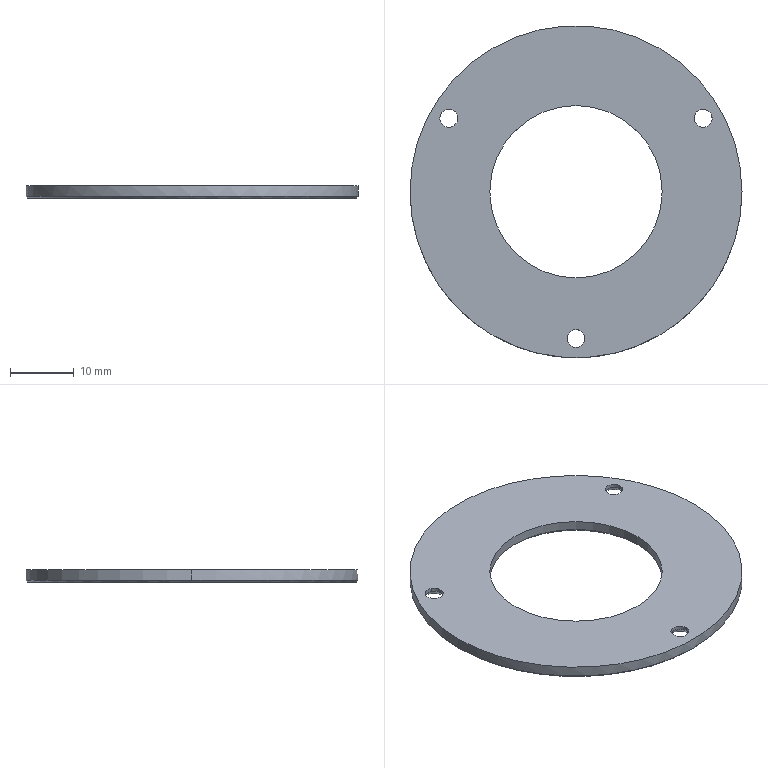Part | STEP file | TCHK-2D-D30-BB-1.stp.STEP | 1 solid | 24 faces | box 52 x 52 x 2 mm | volume 3013 mm3 | cone 12 | cylinder 10 | plane 2 | commonest cylinder face diameters 2.8 x6 27 x2 52 x2
STEP:
#1=CARTESIAN_POINT('',(14.,0.,0.000006287));
#2=VERTEX_POINT('',#1);
#3=CARTESIAN_POINT('',(-14.,0.,0.000006287));
#4=VERTEX_POINT('',#3);
#5=CARTESIAN_POINT('',(0.,0.,0.000006287));
#6=DIRECTION('',(0.,0.,1.));
#7=DIRECTION('',(1.,0.,0.));
#8=AXIS2_PLACEMENT_3D('',#5,#6,#7);
#9=CIRCLE('',#8,14.);
#10=EDGE_CURVE('',#2,#4,#9,.T.);
#11=ORIENTED_EDGE('',*,*,#10,.T.);
#12=CARTESIAN_POINT('',(0.,-14.,0.000006287));
#13=VERTEX_POINT('',#12);
#14=CARTESIAN_POINT('',(0.,0.,0.000006287));
#15=DIRECTION('',(0.,0.,1.));
#16=DIRECTION('',(-1.,0.,0.));
#17=AXIS2_PLACEMENT_3D('',#14,#15,#16);
#18=CIRCLE('',#17,14.);
#19=EDGE_CURVE('',#4,#13,#18,.T.);
#20=ORIENTED_EDGE('',*,*,#19,.T.);
#21=CARTESIAN_POINT('',(0.,0.,0.000006287));
#22=DIRECTION('',(0.,0.,1.));
#23=DIRECTION('',(-1.,0.,0.));
#24=AXIS2_PLACEMENT_3D('',#21,#22,#23);
#25=CIRCLE('',#24,14.);
#26=EDGE_CURVE('',#13,#2,#25,.T.);
#27=ORIENTED_EDGE('',*,*,#26,.T.);
#28=EDGE_LOOP('',(#11,#20,#27));
#29=FACE_BOUND('',#28,.T.);
#30=CARTESIAN_POINT('',(-0.7839,-25.688,0.));
#31=VERTEX_POINT('',#30);
#32=CARTESIAN_POINT('',(-1.4,-25.425,0.));
#33=VERTEX_POINT('',#32);
#34=CARTESIAN_POINT('',(0.,-23.,0.));
#35=DIRECTION('',(0.,0.,-1.));
#36=DIRECTION('',(-0.28,-0.96,0.));
#37=AXIS2_PLACEMENT_3D('',#34,#35,#36);
#38=CIRCLE('',#37,2.8);
#39=EDGE_CURVE('',#31,#33,#38,.T.);
#40=ORIENTED_EDGE('',*,*,#39,.F.);
#41=CARTESIAN_POINT('',(-25.7,-0.000000004,0.000001018));
#42=VERTEX_POINT('',#41);
#43=CARTESIAN_POINT('',(0.,0.,0.));
#44=DIRECTION('',(0.,0.,-1.));
#45=DIRECTION('',(-0.0305,-0.9995,0.));
#46=AXIS2_PLACEMENT_3D('',#43,#44,#45);
#47=CIRCLE('',#46,25.7);
#48=EDGE_CURVE('',#31,#42,#47,.T.);
#49=ORIENTED_EDGE('',*,*,#48,.T.);
#50=CARTESIAN_POINT('',(-22.638,12.165,0.));
#51=VERTEX_POINT('',#50);
#52=CARTESIAN_POINT('',(0.,0.,0.));
#53=DIRECTION('',(0.,0.,-1.));
#54=DIRECTION('',(-1.,0.,0.));
#55=AXIS2_PLACEMENT_3D('',#52,#53,#54);
#56=CIRCLE('',#55,25.7);
#57=EDGE_CURVE('',#42,#51,#56,.T.);
#58=ORIENTED_EDGE('',*,*,#57,.T.);
#59=CARTESIAN_POINT('',(-18.519,9.075,0.));
#60=VERTEX_POINT('',#59);
#61=CARTESIAN_POINT('',(-19.919,11.5,0.));
#62=DIRECTION('',(0.,0.,-1.));
#63=DIRECTION('',(0.5,-0.866,0.));
#64=AXIS2_PLACEMENT_3D('',#61,#62,#63);
#65=CIRCLE('',#64,2.8);
#66=EDGE_CURVE('',#60,#51,#65,.T.);
#67=ORIENTED_EDGE('',*,*,#66,.F.);
#68=CARTESIAN_POINT('',(-21.319,13.925,0.));
#69=VERTEX_POINT('',#68);
#70=CARTESIAN_POINT('',(-19.919,11.5,0.));
#71=DIRECTION('',(0.,0.,-1.));
#72=DIRECTION('',(-0.5,0.866,0.));
#73=AXIS2_PLACEMENT_3D('',#70,#71,#72);
#74=CIRCLE('',#73,2.8);
#75=EDGE_CURVE('',#69,#60,#74,.T.);
#76=ORIENTED_EDGE('',*,*,#75,.F.);
#77=CARTESIAN_POINT('',(-21.855,13.523,0.));
#78=VERTEX_POINT('',#77);
#79=CARTESIAN_POINT('',(-19.919,11.5,0.));
#80=DIRECTION('',(0.,0.,-1.));
#81=DIRECTION('',(-0.6914,0.7225,0.));
#82=AXIS2_PLACEMENT_3D('',#79,#80,#81);
#83=CIRCLE('',#82,2.8);
#84=EDGE_CURVE('',#78,#69,#83,.T.);
#85=ORIENTED_EDGE('',*,*,#84,.F.);
#86=CARTESIAN_POINT('',(21.855,13.523,0.));
#87=VERTEX_POINT('',#86);
#88=CARTESIAN_POINT('',(0.,0.,0.));
#89=DIRECTION('',(0.,0.,-1.));
#90=DIRECTION('',(-0.8504,0.5262,0.));
#91=AXIS2_PLACEMENT_3D('',#88,#89,#90);
#92=CIRCLE('',#91,25.7);
#93=EDGE_CURVE('',#78,#87,#92,.T.);
#94=ORIENTED_EDGE('',*,*,#93,.T.);
#95=CARTESIAN_POINT('',(17.119,11.5,0.));
#96=VERTEX_POINT('',#95);
#97=CARTESIAN_POINT('',(19.919,11.5,0.));
#98=DIRECTION('',(0.,0.,-1.));
#99=DIRECTION('',(-1.,0.,0.));
#100=AXIS2_PLACEMENT_3D('',#97,#98,#99);
#101=CIRCLE('',#100,2.8);
#102=EDGE_CURVE('',#96,#87,#101,.T.);
#103=ORIENTED_EDGE('',*,*,#102,.F.);
#104=CARTESIAN_POINT('',(22.719,11.5,0.));
#105=VERTEX_POINT('',#104);
#106=CARTESIAN_POINT('',(19.919,11.5,0.));
#107=DIRECTION('',(0.,0.,-1.));
#108=DIRECTION('',(1.,0.,0.));
#109=AXIS2_PLACEMENT_3D('',#106,#107,#108);
#110=CIRCLE('',#109,2.8);
#111=EDGE_CURVE('',#105,#96,#110,.T.);
#112=ORIENTED_EDGE('',*,*,#111,.F.);
#113=CARTESIAN_POINT('',(22.638,12.165,0.));
#114=VERTEX_POINT('',#113);
#115=CARTESIAN_POINT('',(19.919,11.5,0.));
#116=DIRECTION('',(0.,0.,-1.));
#117=DIRECTION('',(0.9714,0.2376,0.));
#118=AXIS2_PLACEMENT_3D('',#115,#116,#117);
#119=CIRCLE('',#118,2.8);
#120=EDGE_CURVE('',#114,#105,#119,.T.);
#121=ORIENTED_EDGE('',*,*,#120,.F.);
#122=CARTESIAN_POINT('',(25.7,0.000000004,0.000001018));
#123=VERTEX_POINT('',#122);
#124=CARTESIAN_POINT('',(0.,0.,0.));
#125=DIRECTION('',(0.,0.,-1.));
#126=DIRECTION('',(0.8809,0.4734,0.));
#127=AXIS2_PLACEMENT_3D('',#124,#125,#126);
#128=CIRCLE('',#127,25.7);
#129=EDGE_CURVE('',#114,#123,#128,.T.);
#130=ORIENTED_EDGE('',*,*,#129,.T.);
#131=CARTESIAN_POINT('',(0.7839,-25.688,0.));
#132=VERTEX_POINT('',#131);
#133=CARTESIAN_POINT('',(0.,0.,0.));
#134=DIRECTION('',(0.,0.,-1.));
#135=DIRECTION('',(1.,0.,0.));
#136=AXIS2_PLACEMENT_3D('',#133,#134,#135);
#137=CIRCLE('',#136,25.7);
#138=EDGE_CURVE('',#123,#132,#137,.T.);
#139=ORIENTED_EDGE('',*,*,#138,.T.);
#140=CARTESIAN_POINT('',(1.4,-20.575,0.));
#141=VERTEX_POINT('',#140);
#142=CARTESIAN_POINT('',(0.,-23.,0.));
#143=DIRECTION('',(0.,0.,-1.));
#144=DIRECTION('',(0.5,0.866,0.));
#145=AXIS2_PLACEMENT_3D('',#142,#143,#144);
#146=CIRCLE('',#145,2.8);
#147=EDGE_CURVE('',#141,#132,#146,.T.);
#148=ORIENTED_EDGE('',*,*,#147,.F.);
#149=CARTESIAN_POINT('',(0.,-23.,0.));
#150=DIRECTION('',(0.,0.,-1.));
#151=DIRECTION('',(-0.5,-0.866,0.));
#152=AXIS2_PLACEMENT_3D('',#149,#150,#151);
#153=CIRCLE('',#152,2.8);
#154=EDGE_CURVE('',#33,#141,#153,.T.);
#155=ORIENTED_EDGE('',*,*,#154,.F.);
#156=EDGE_LOOP('',(#40,#49,#58,#67,#76,#85,#94,#103,#112,#121,#130,#139,#148,#155));
#157=FACE_OUTER_BOUND('',#156,.T.);
#158=CARTESIAN_POINT('',(0.,0.,0.));
#159=DIRECTION('',(0.,0.,1.));
#160=DIRECTION('',(1.,0.,0.));
#161=AXIS2_PLACEMENT_3D('',#158,#159,#160);
#162=PLANE('',#161);
#163=ADVANCED_FACE('',(#29,#157),#162,.F.);
#164=CARTESIAN_POINT('',(0.,-13.5,0.5));
#165=VERTEX_POINT('',#164);
#166=CARTESIAN_POINT('',(0.,-13.75,0.25));
#167=DIRECTION('',(0.,-0.7071,-0.7071));
#168=VECTOR('',#167,1000.);
#169=LINE('',#166,#168);
#170=EDGE_CURVE('',#165,#13,#169,.T.);
#171=ORIENTED_EDGE('',*,*,#170,.F.);
#172=CARTESIAN_POINT('',(13.5,0.,0.5));
#173=VERTEX_POINT('',#172);
#174=CARTESIAN_POINT('',(0.,0.,0.5));
#175=DIRECTION('',(0.,0.,1.));
#176=DIRECTION('',(-1.,0.,0.));
#177=AXIS2_PLACEMENT_3D('',#174,#175,#176);
#178=CIRCLE('',#177,13.5);
#179=EDGE_CURVE('',#165,#173,#178,.T.);
#180=ORIENTED_EDGE('',*,*,#179,.T.);
#181=CARTESIAN_POINT('',(14.,0.000000008,0.000002614));
#182=DIRECTION('',(-0.7071,-0.000000003,0.7071));
#183=VECTOR('',#182,1000.);
#184=LINE('',#181,#183);
#185=EDGE_CURVE('',#2,#173,#184,.T.);
#186=ORIENTED_EDGE('',*,*,#185,.F.);
#187=ORIENTED_EDGE('',*,*,#26,.F.);
#188=EDGE_LOOP('',(#171,#180,#186,#187));
#189=FACE_OUTER_BOUND('',#188,.T.);
#190=CARTESIAN_POINT('',(0.,0.,0.25));
#191=DIRECTION('',(0.,0.,-1.));
#192=DIRECTION('',(0.,-1.,0.));
#193=AXIS2_PLACEMENT_3D('',#190,#191,#192);
#194=CONICAL_SURFACE('',#193,13.75,0.7854);
#195=ADVANCED_FACE('',(#189),#194,.F.);
#196=ORIENTED_EDGE('',*,*,#185,.T.);
#197=CARTESIAN_POINT('',(-13.5,0.,0.5));
#198=VERTEX_POINT('',#197);
#199=CARTESIAN_POINT('',(0.,0.,0.5));
#200=DIRECTION('',(0.,0.,1.));
#201=DIRECTION('',(1.,0.,0.));
#202=AXIS2_PLACEMENT_3D('',#199,#200,#201);
#203=CIRCLE('',#202,13.5);
#204=EDGE_CURVE('',#173,#198,#203,.T.);
#205=ORIENTED_EDGE('',*,*,#204,.T.);
#206=CARTESIAN_POINT('',(-14.,-0.000000008,0.000002614));
#207=DIRECTION('',(0.7071,0.000000003,0.7071));
#208=VECTOR('',#207,1000.);
#209=LINE('',#206,#208);
#210=EDGE_CURVE('',#4,#198,#209,.T.);
#211=ORIENTED_EDGE('',*,*,#210,.F.);
#212=ORIENTED_EDGE('',*,*,#10,.F.);
#213=EDGE_LOOP('',(#196,#205,#211,#212));
#214=FACE_OUTER_BOUND('',#213,.T.);
#215=CARTESIAN_POINT('',(0.,0.,0.25));
#216=DIRECTION('',(0.,0.,-1.));
#217=DIRECTION('',(0.,-1.,0.));
#218=AXIS2_PLACEMENT_3D('',#215,#216,#217);
#219=CONICAL_SURFACE('',#218,13.75,0.7854);
#220=ADVANCED_FACE('',(#214),#219,.F.);
#221=CARTESIAN_POINT('',(13.5,0.,2.));
#222=VERTEX_POINT('',#221);
#223=CARTESIAN_POINT('',(13.5,0.,2.));
#224=DIRECTION('',(0.00000126,0.000000004,-1.));
#225=VECTOR('',#224,1000.);
#226=LINE('',#223,#225);
#227=EDGE_CURVE('',#222,#173,#226,.T.);
#228=ORIENTED_EDGE('',*,*,#227,.F.);
#229=CARTESIAN_POINT('',(-13.5,0.,2.));
#230=VERTEX_POINT('',#229);
#231=CARTESIAN_POINT('',(0.,0.,2.));
#232=DIRECTION('',(0.,0.,1.));
#233=DIRECTION('',(1.,0.,0.));
#234=AXIS2_PLACEMENT_3D('',#231,#232,#233);
#235=CIRCLE('',#234,13.5);
#236=EDGE_CURVE('',#222,#230,#235,.T.);
#237=ORIENTED_EDGE('',*,*,#236,.T.);
#238=CARTESIAN_POINT('',(-13.5,0.,2.));
#239=DIRECTION('',(-0.00000126,-0.000000004,-1.));
#240=VECTOR('',#239,1000.);
#241=LINE('',#238,#240);
#242=EDGE_CURVE('',#230,#198,#241,.T.);
#243=ORIENTED_EDGE('',*,*,#242,.T.);
#244=ORIENTED_EDGE('',*,*,#204,.F.);
#245=EDGE_LOOP('',(#228,#237,#243,#244));
#246=FACE_OUTER_BOUND('',#245,.T.);
#247=CARTESIAN_POINT('',(0.,0.,2.));
#248=DIRECTION('',(0.,0.,1.));
#249=DIRECTION('',(1.,0.,0.));
#250=AXIS2_PLACEMENT_3D('',#247,#248,#249);
#251=CYLINDRICAL_SURFACE('',#250,13.5);
#252=ADVANCED_FACE('',(#246),#251,.F.);
#253=ORIENTED_EDGE('',*,*,#242,.F.);
#254=CARTESIAN_POINT('',(0.,0.,2.));
#255=DIRECTION('',(0.,0.,1.));
#256=DIRECTION('',(-1.,0.,0.));
#257=AXIS2_PLACEMENT_3D('',#254,#255,#256);
#258=CIRCLE('',#257,13.5);
#259=EDGE_CURVE('',#230,#222,#258,.T.);
#260=ORIENTED_EDGE('',*,*,#259,.T.);
#261=ORIENTED_EDGE('',*,*,#227,.T.);
#262=ORIENTED_EDGE('',*,*,#179,.F.);
#263=CARTESIAN_POINT('',(0.,0.,0.5));
#264=DIRECTION('',(0.,0.,1.));
#265=DIRECTION('',(-1.,0.,0.));
#266=AXIS2_PLACEMENT_3D('',#263,#264,#265);
#267=CIRCLE('',#266,13.5);
#268=EDGE_CURVE('',#198,#165,#267,.T.);
#269=ORIENTED_EDGE('',*,*,#268,.F.);
#270=EDGE_LOOP('',(#253,#260,#261,#262,#269));
#271=FACE_OUTER_BOUND('',#270,.T.);
#272=CARTESIAN_POINT('',(0.,0.,2.));
#273=DIRECTION('',(0.,0.,1.));
#274=DIRECTION('',(1.,0.,0.));
#275=AXIS2_PLACEMENT_3D('',#272,#273,#274);
#276=CYLINDRICAL_SURFACE('',#275,13.5);
#277=ADVANCED_FACE('',(#271),#276,.F.);
#278=CARTESIAN_POINT('',(1.4,-23.,2.));
#279=VERTEX_POINT('',#278);
#280=CARTESIAN_POINT('',(-1.4,-23.,2.));
#281=VERTEX_POINT('',#280);
#282=CARTESIAN_POINT('',(0.,-23.,2.));
#283=DIRECTION('',(0.,0.,-1.));
#284=DIRECTION('',(1.,0.,0.));
#285=AXIS2_PLACEMENT_3D('',#282,#283,#284);
#286=CIRCLE('',#285,1.4);
#287=EDGE_CURVE('',#279,#281,#286,.T.);
#288=ORIENTED_EDGE('',*,*,#287,.T.);
#289=CARTESIAN_POINT('',(0.,-23.,2.));
#290=DIRECTION('',(0.,0.,-1.));
#291=DIRECTION('',(-1.,0.,0.));
#292=AXIS2_PLACEMENT_3D('',#289,#290,#291);
#293=CIRCLE('',#292,1.4);
#294=EDGE_CURVE('',#281,#279,#293,.T.);
#295=ORIENTED_EDGE('',*,*,#294,.T.);
#296=EDGE_LOOP('',(#288,#295));
#297=FACE_BOUND('',#296,.T.);
#298=CARTESIAN_POINT('',(19.219,12.712,2.));
#299=VERTEX_POINT('',#298);
#300=CARTESIAN_POINT('',(20.619,10.288,2.));
#301=VERTEX_POINT('',#300);
#302=CARTESIAN_POINT('',(19.919,11.5,2.));
#303=DIRECTION('',(0.,0.,-1.));
#304=DIRECTION('',(-0.5,0.866,0.));
#305=AXIS2_PLACEMENT_3D('',#302,#303,#304);
#306=CIRCLE('',#305,1.4);
#307=EDGE_CURVE('',#299,#301,#306,.T.);
#308=ORIENTED_EDGE('',*,*,#307,.T.);
#309=CARTESIAN_POINT('',(19.919,11.5,2.));
#310=DIRECTION('',(0.,0.,-1.));
#311=DIRECTION('',(0.5,-0.866,0.));
#312=AXIS2_PLACEMENT_3D('',#309,#310,#311);
#313=CIRCLE('',#312,1.4);
#314=EDGE_CURVE('',#301,#299,#313,.T.);
#315=ORIENTED_EDGE('',*,*,#314,.T.);
#316=EDGE_LOOP('',(#308,#315));
#317=FACE_BOUND('',#316,.T.);
#318=CARTESIAN_POINT('',(-20.619,10.288,2.));
#319=VERTEX_POINT('',#318);
#320=CARTESIAN_POINT('',(-19.219,12.712,2.));
#321=VERTEX_POINT('',#320);
#322=CARTESIAN_POINT('',(-19.919,11.5,2.));
#323=DIRECTION('',(0.,0.,-1.));
#324=DIRECTION('',(-0.5,-0.866,0.));
#325=AXIS2_PLACEMENT_3D('',#322,#323,#324);
#326=CIRCLE('',#325,1.4);
#327=EDGE_CURVE('',#319,#321,#326,.T.);
#328=ORIENTED_EDGE('',*,*,#327,.T.);
#329=CARTESIAN_POINT('',(-19.919,11.5,2.));
#330=DIRECTION('',(0.,0.,-1.));
#331=DIRECTION('',(0.5,0.866,0.));
#332=AXIS2_PLACEMENT_3D('',#329,#330,#331);
#333=CIRCLE('',#332,1.4);
#334=EDGE_CURVE('',#321,#319,#333,.T.);
#335=ORIENTED_EDGE('',*,*,#334,.T.);
#336=EDGE_LOOP('',(#328,#335));
#337=FACE_BOUND('',#336,.T.);
#338=ORIENTED_EDGE('',*,*,#259,.F.);
#339=ORIENTED_EDGE('',*,*,#236,.F.);
#340=EDGE_LOOP('',(#338,#339));
#341=FACE_BOUND('',#340,.T.);
#342=CARTESIAN_POINT('',(-26.,0.,2.));
#343=VERTEX_POINT('',#342);
#344=CARTESIAN_POINT('',(26.,0.,2.));
#345=VERTEX_POINT('',#344);
#346=CARTESIAN_POINT('',(0.,0.,2.));
#347=DIRECTION('',(0.,0.,1.));
#348=DIRECTION('',(-1.,0.,0.));
#349=AXIS2_PLACEMENT_3D('',#346,#347,#348);
#350=CIRCLE('',#349,26.);
#351=EDGE_CURVE('',#343,#345,#350,.T.);
#352=ORIENTED_EDGE('',*,*,#351,.T.);
#353=CARTESIAN_POINT('',(0.,0.,2.));
#354=DIRECTION('',(0.,0.,1.));
#355=DIRECTION('',(1.,0.,0.));
#356=AXIS2_PLACEMENT_3D('',#353,#354,#355);
#357=CIRCLE('',#356,26.);
#358=EDGE_CURVE('',#345,#343,#357,.T.);
#359=ORIENTED_EDGE('',*,*,#358,.T.);
#360=EDGE_LOOP('',(#352,#359));
#361=FACE_OUTER_BOUND('',#360,.T.);
#362=CARTESIAN_POINT('',(0.,0.,2.));
#363=DIRECTION('',(0.,0.,1.));
#364=DIRECTION('',(1.,0.,0.));
#365=AXIS2_PLACEMENT_3D('',#362,#363,#364);
#366=PLANE('',#365);
#367=ADVANCED_FACE('',(#297,#317,#337,#341,#361),#366,.T.);
#368=CARTESIAN_POINT('',(-26.,0.,0.3));
#369=VERTEX_POINT('',#368);
#370=CARTESIAN_POINT('',(-26.,-0.000000003,0.3));
#371=DIRECTION('',(-0.000000455,0.000000002,1.));
#372=VECTOR('',#371,1000.);
#373=LINE('',#370,#372);
#374=EDGE_CURVE('',#369,#343,#373,.T.);
#375=ORIENTED_EDGE('',*,*,#374,.T.);
#376=ORIENTED_EDGE('',*,*,#358,.F.);
#377=CARTESIAN_POINT('',(26.,0.,0.3));
#378=VERTEX_POINT('',#377);
#379=CARTESIAN_POINT('',(26.,0.000000003,0.3));
#380=DIRECTION('',(0.000000455,-0.000000002,1.));
#381=VECTOR('',#380,1000.);
#382=LINE('',#379,#381);
#383=EDGE_CURVE('',#378,#345,#382,.T.);
#384=ORIENTED_EDGE('',*,*,#383,.F.);
#385=CARTESIAN_POINT('',(0.,0.,0.3));
#386=DIRECTION('',(0.,0.,-1.));
#387=DIRECTION('',(-1.,0.,0.));
#388=AXIS2_PLACEMENT_3D('',#385,#386,#387);
#389=CIRCLE('',#388,26.);
#390=EDGE_CURVE('',#369,#378,#389,.T.);
#391=ORIENTED_EDGE('',*,*,#390,.F.);
#392=EDGE_LOOP('',(#375,#376,#384,#391));
#393=FACE_OUTER_BOUND('',#392,.T.);
#394=CARTESIAN_POINT('',(0.,0.,0.));
#395=DIRECTION('',(0.,0.,1.));
#396=DIRECTION('',(1.,0.,0.));
#397=AXIS2_PLACEMENT_3D('',#394,#395,#396);
#398=CYLINDRICAL_SURFACE('',#397,26.);
#399=ADVANCED_FACE('',(#393),#398,.T.);
#400=ORIENTED_EDGE('',*,*,#57,.F.);
#401=CARTESIAN_POINT('',(-25.7,-0.000000004,0.000001018));
#402=DIRECTION('',(-0.7071,0.000000002,0.7071));
#403=VECTOR('',#402,1000.);
#404=LINE('',#401,#403);
#405=EDGE_CURVE('',#42,#369,#404,.T.);
#406=ORIENTED_EDGE('',*,*,#405,.T.);
#407=ORIENTED_EDGE('',*,*,#390,.T.);
#408=CARTESIAN_POINT('',(25.7,0.000000004,0.000001018));
#409=DIRECTION('',(0.7071,-0.000000002,0.7071));
#410=VECTOR('',#409,1000.);
#411=LINE('',#408,#410);
#412=EDGE_CURVE('',#123,#378,#411,.T.);
#413=ORIENTED_EDGE('',*,*,#412,.F.);
#414=ORIENTED_EDGE('',*,*,#129,.F.);
#415=CARTESIAN_POINT('',(22.638,12.165,0.));
#416=CARTESIAN_POINT('',(22.45,12.657,0.06653));
#417=CARTESIAN_POINT('',(22.186,13.113,0.06653));
#418=CARTESIAN_POINT('',(21.855,13.523,0.));
#419=B_SPLINE_CURVE_WITH_KNOTS('',3,(#415,#416,#417,#418),.UNSPECIFIED.,.F.,.F.,(4,4),(0.,1.),.UNSPECIFIED.);
#420=EDGE_CURVE('',#114,#87,#419,.T.);
#421=ORIENTED_EDGE('',*,*,#420,.T.);
#422=ORIENTED_EDGE('',*,*,#93,.F.);
#423=CARTESIAN_POINT('',(-21.855,13.523,0.));
#424=CARTESIAN_POINT('',(-22.186,13.113,0.06653));
#425=CARTESIAN_POINT('',(-22.45,12.657,0.06653));
#426=CARTESIAN_POINT('',(-22.638,12.165,0.));
#427=B_SPLINE_CURVE_WITH_KNOTS('',3,(#423,#424,#425,#426),.UNSPECIFIED.,.F.,.F.,(4,4),(0.,1.),.UNSPECIFIED.);
#428=EDGE_CURVE('',#78,#51,#427,.T.);
#429=ORIENTED_EDGE('',*,*,#428,.T.);
#430=EDGE_LOOP('',(#400,#406,#407,#413,#414,#421,#422,#429));
#431=FACE_OUTER_BOUND('',#430,.T.);
#432=CARTESIAN_POINT('',(0.,0.,0.15));
#433=DIRECTION('',(0.,0.,1.));
#434=DIRECTION('',(0.,-1.,0.));
#435=AXIS2_PLACEMENT_3D('',#432,#433,#434);
#436=CONICAL_SURFACE('',#435,25.85,0.7854);
#437=ADVANCED_FACE('',(#431),#436,.T.);
#438=ORIENTED_EDGE('',*,*,#428,.F.);
#439=ORIENTED_EDGE('',*,*,#84,.T.);
#440=CARTESIAN_POINT('',(-20.619,12.712,1.4));
#441=VERTEX_POINT('',#440);
#442=CARTESIAN_POINT('',(-21.319,13.925,0.));
#443=DIRECTION('',(0.3536,-0.6124,0.7071));
#444=VECTOR('',#443,1000.);
#445=LINE('',#442,#444);
#446=EDGE_CURVE('',#69,#441,#445,.T.);
#447=ORIENTED_EDGE('',*,*,#446,.T.);
#448=CARTESIAN_POINT('',(-20.619,10.288,1.4));
#449=VERTEX_POINT('',#448);
#450=CARTESIAN_POINT('',(-19.919,11.5,1.4));
#451=DIRECTION('',(0.,0.,-1.));
#452=DIRECTION('',(-0.5,-0.866,0.));
#453=AXIS2_PLACEMENT_3D('',#450,#451,#452);
#454=CIRCLE('',#453,1.4);
#455=EDGE_CURVE('',#449,#441,#454,.T.);
#456=ORIENTED_EDGE('',*,*,#455,.F.);
#457=CARTESIAN_POINT('',(-19.219,10.288,1.4));
#458=VERTEX_POINT('',#457);
#459=CARTESIAN_POINT('',(-19.919,11.5,1.4));
#460=DIRECTION('',(0.,0.,-1.));
#461=DIRECTION('',(0.5,-0.866,0.));
#462=AXIS2_PLACEMENT_3D('',#459,#460,#461);
#463=CIRCLE('',#462,1.4);
#464=EDGE_CURVE('',#458,#449,#463,.T.);
#465=ORIENTED_EDGE('',*,*,#464,.F.);
#466=CARTESIAN_POINT('',(-18.519,9.075,0.));
#467=DIRECTION('',(-0.3536,0.6124,0.7071));
#468=VECTOR('',#467,1000.);
#469=LINE('',#466,#468);
#470=EDGE_CURVE('',#60,#458,#469,.T.);
#471=ORIENTED_EDGE('',*,*,#470,.F.);
#472=ORIENTED_EDGE('',*,*,#66,.T.);
#473=EDGE_LOOP('',(#438,#439,#447,#456,#465,#471,#472));
#474=FACE_OUTER_BOUND('',#473,.T.);
#475=CARTESIAN_POINT('',(-19.919,11.5,0.7));
#476=DIRECTION('',(0.,0.,-1.));
#477=DIRECTION('',(0.5,-0.866,0.));
#478=AXIS2_PLACEMENT_3D('',#475,#476,#477);
#479=CONICAL_SURFACE('',#478,2.1,0.7854);
#480=ADVANCED_FACE('',(#474),#479,.F.);
#481=ORIENTED_EDGE('',*,*,#470,.T.);
#482=CARTESIAN_POINT('',(-19.219,12.712,1.4));
#483=VERTEX_POINT('',#482);
#484=CARTESIAN_POINT('',(-19.919,11.5,1.4));
#485=DIRECTION('',(0.,0.,-1.));
#486=DIRECTION('',(0.5,0.866,0.));
#487=AXIS2_PLACEMENT_3D('',#484,#485,#486);
#488=CIRCLE('',#487,1.4);
#489=EDGE_CURVE('',#483,#458,#488,.T.);
#490=ORIENTED_EDGE('',*,*,#489,.F.);
#491=CARTESIAN_POINT('',(-19.919,11.5,1.4));
#492=DIRECTION('',(0.,0.,-1.));
#493=DIRECTION('',(-0.5,0.866,0.));
#494=AXIS2_PLACEMENT_3D('',#491,#492,#493);
#495=CIRCLE('',#494,1.4);
#496=EDGE_CURVE('',#441,#483,#495,.T.);
#497=ORIENTED_EDGE('',*,*,#496,.F.);
#498=ORIENTED_EDGE('',*,*,#446,.F.);
#499=ORIENTED_EDGE('',*,*,#75,.T.);
#500=EDGE_LOOP('',(#481,#490,#497,#498,#499));
#501=FACE_OUTER_BOUND('',#500,.T.);
#502=CARTESIAN_POINT('',(-19.919,11.5,0.7));
#503=DIRECTION('',(0.,0.,-1.));
#504=DIRECTION('',(0.5,-0.866,0.));
#505=AXIS2_PLACEMENT_3D('',#502,#503,#504);
#506=CONICAL_SURFACE('',#505,2.1,0.7854);
#507=ADVANCED_FACE('',(#501),#506,.F.);
#508=CARTESIAN_POINT('',(-19.219,12.712,2.));
#509=DIRECTION('',(0.,0.,-1.));
#510=VECTOR('',#509,1000.);
#511=LINE('',#508,#510);
#512=EDGE_CURVE('',#321,#483,#511,.T.);
#513=ORIENTED_EDGE('',*,*,#512,.F.);
#514=ORIENTED_EDGE('',*,*,#327,.F.);
#515=CARTESIAN_POINT('',(-20.619,10.288,2.));
#516=DIRECTION('',(0.,0.,-1.));
#517=VECTOR('',#516,1000.);
#518=LINE('',#515,#517);
#519=EDGE_CURVE('',#319,#449,#518,.T.);
#520=ORIENTED_EDGE('',*,*,#519,.T.);
#521=ORIENTED_EDGE('',*,*,#455,.T.);
#522=ORIENTED_EDGE('',*,*,#496,.T.);
#523=EDGE_LOOP('',(#513,#514,#520,#521,#522));
#524=FACE_OUTER_BOUND('',#523,.T.);
#525=CARTESIAN_POINT('',(-19.919,11.5,2.));
#526=DIRECTION('',(0.,0.,-1.));
#527=DIRECTION('',(0.5,0.866,0.));
#528=AXIS2_PLACEMENT_3D('',#525,#526,#527);
#529=CYLINDRICAL_SURFACE('',#528,1.4);
#530=ADVANCED_FACE('',(#524),#529,.F.);
#531=ORIENTED_EDGE('',*,*,#464,.T.);
#532=ORIENTED_EDGE('',*,*,#519,.F.);
#533=ORIENTED_EDGE('',*,*,#334,.F.);
#534=ORIENTED_EDGE('',*,*,#512,.T.);
#535=ORIENTED_EDGE('',*,*,#489,.T.);
#536=EDGE_LOOP('',(#531,#532,#533,#534,#535));
#537=FACE_OUTER_BOUND('',#536,.T.);
#538=CARTESIAN_POINT('',(-19.919,11.5,2.));
#539=DIRECTION('',(0.,0.,-1.));
#540=DIRECTION('',(0.5,0.866,0.));
#541=AXIS2_PLACEMENT_3D('',#538,#539,#540);
#542=CYLINDRICAL_SURFACE('',#541,1.4);
#543=ADVANCED_FACE('',(#537),#542,.F.);
#544=ORIENTED_EDGE('',*,*,#420,.F.);
#545=ORIENTED_EDGE('',*,*,#120,.T.);
#546=CARTESIAN_POINT('',(21.319,11.5,1.4));
#547=VERTEX_POINT('',#546);
#548=CARTESIAN_POINT('',(22.719,11.5,0.));
#549=DIRECTION('',(-0.7071,0.,0.7071));
#550=VECTOR('',#549,1000.);
#551=LINE('',#548,#550);
#552=EDGE_CURVE('',#105,#547,#551,.T.);
#553=ORIENTED_EDGE('',*,*,#552,.T.);
#554=CARTESIAN_POINT('',(19.219,12.712,1.4));
#555=VERTEX_POINT('',#554);
#556=CARTESIAN_POINT('',(19.919,11.5,1.4));
#557=DIRECTION('',(0.,0.,-1.));
#558=DIRECTION('',(-0.5,0.866,0.));
#559=AXIS2_PLACEMENT_3D('',#556,#557,#558);
#560=CIRCLE('',#559,1.4);
#561=EDGE_CURVE('',#555,#547,#560,.T.);
#562=ORIENTED_EDGE('',*,*,#561,.F.);
#563=CARTESIAN_POINT('',(18.519,11.5,1.4));
#564=VERTEX_POINT('',#563);
#565=CARTESIAN_POINT('',(19.919,11.5,1.4));
#566=DIRECTION('',(0.,0.,-1.));
#567=DIRECTION('',(-1.,0.,0.));
#568=AXIS2_PLACEMENT_3D('',#565,#566,#567);
#569=CIRCLE('',#568,1.4);
#570=EDGE_CURVE('',#564,#555,#569,.T.);
#571=ORIENTED_EDGE('',*,*,#570,.F.);
#572=CARTESIAN_POINT('',(17.119,11.5,0.));
#573=DIRECTION('',(0.7071,0.,0.7071));
#574=VECTOR('',#573,1000.);
#575=LINE('',#572,#574);
#576=EDGE_CURVE('',#96,#564,#575,.T.);
#577=ORIENTED_EDGE('',*,*,#576,.F.);
#578=ORIENTED_EDGE('',*,*,#102,.T.);
#579=EDGE_LOOP('',(#544,#545,#553,#562,#571,#577,#578));
#580=FACE_OUTER_BOUND('',#579,.T.);
#581=CARTESIAN_POINT('',(19.919,11.5,0.7));
#582=DIRECTION('',(0.,0.,-1.));
#583=DIRECTION('',(-1.,0.,0.));
#584=AXIS2_PLACEMENT_3D('',#581,#582,#583);
#585=CONICAL_SURFACE('',#584,2.1,0.7854);
#586=ADVANCED_FACE('',(#580),#585,.F.);
#587=ORIENTED_EDGE('',*,*,#576,.T.);
#588=CARTESIAN_POINT('',(20.619,10.288,1.4));
#589=VERTEX_POINT('',#588);
#590=CARTESIAN_POINT('',(19.919,11.5,1.4));
#591=DIRECTION('',(0.,0.,-1.));
#592=DIRECTION('',(0.5,-0.866,0.));
#593=AXIS2_PLACEMENT_3D('',#590,#591,#592);
#594=CIRCLE('',#593,1.4);
#595=EDGE_CURVE('',#589,#564,#594,.T.);
#596=ORIENTED_EDGE('',*,*,#595,.F.);
#597=CARTESIAN_POINT('',(19.919,11.5,1.4));
#598=DIRECTION('',(0.,0.,-1.));
#599=DIRECTION('',(1.,0.,0.));
#600=AXIS2_PLACEMENT_3D('',#597,#598,#599);
#601=CIRCLE('',#600,1.4);
#602=EDGE_CURVE('',#547,#589,#601,.T.);
#603=ORIENTED_EDGE('',*,*,#602,.F.);
#604=ORIENTED_EDGE('',*,*,#552,.F.);
#605=ORIENTED_EDGE('',*,*,#111,.T.);
#606=EDGE_LOOP('',(#587,#596,#603,#604,#605));
#607=FACE_OUTER_BOUND('',#606,.T.);
#608=CARTESIAN_POINT('',(19.919,11.5,0.7));
#609=DIRECTION('',(0.,0.,-1.));
#610=DIRECTION('',(-1.,0.,0.));
#611=AXIS2_PLACEMENT_3D('',#608,#609,#610);
#612=CONICAL_SURFACE('',#611,2.1,0.7854);
#613=ADVANCED_FACE('',(#607),#612,.F.);
#614=CARTESIAN_POINT('',(20.619,10.288,2.));
#615=DIRECTION('',(0.,0.,-1.));
#616=VECTOR('',#615,1000.);
#617=LINE('',#614,#616);
#618=EDGE_CURVE('',#301,#589,#617,.T.);
#619=ORIENTED_EDGE('',*,*,#618,.F.);
#620=ORIENTED_EDGE('',*,*,#307,.F.);
#621=CARTESIAN_POINT('',(19.219,12.712,2.));
#622=DIRECTION('',(0.,0.,-1.));
#623=VECTOR('',#622,1000.);
#624=LINE('',#621,#623);
#625=EDGE_CURVE('',#299,#555,#624,.T.);
#626=ORIENTED_EDGE('',*,*,#625,.T.);
#627=ORIENTED_EDGE('',*,*,#561,.T.);
#628=ORIENTED_EDGE('',*,*,#602,.T.);
#629=EDGE_LOOP('',(#619,#620,#626,#627,#628));
#630=FACE_OUTER_BOUND('',#629,.T.);
#631=CARTESIAN_POINT('',(19.919,11.5,2.));
#632=DIRECTION('',(0.,0.,-1.));
#633=DIRECTION('',(0.5,-0.866,0.));
#634=AXIS2_PLACEMENT_3D('',#631,#632,#633);
#635=CYLINDRICAL_SURFACE('',#634,1.4);
#636=ADVANCED_FACE('',(#630),#635,.F.);
#637=ORIENTED_EDGE('',*,*,#570,.T.);
#638=ORIENTED_EDGE('',*,*,#625,.F.);
#639=ORIENTED_EDGE('',*,*,#314,.F.);
#640=ORIENTED_EDGE('',*,*,#618,.T.);
#641=ORIENTED_EDGE('',*,*,#595,.T.);
#642=EDGE_LOOP('',(#637,#638,#639,#640,#641));
#643=FACE_OUTER_BOUND('',#642,.T.);
#644=CARTESIAN_POINT('',(19.919,11.5,2.));
#645=DIRECTION('',(0.,0.,-1.));
#646=DIRECTION('',(0.5,-0.866,0.));
#647=AXIS2_PLACEMENT_3D('',#644,#645,#646);
#648=CYLINDRICAL_SURFACE('',#647,1.4);
#649=ADVANCED_FACE('',(#643),#648,.F.);
#650=CARTESIAN_POINT('',(0.000000009,-25.75,0.05));
#651=VERTEX_POINT('',#650);
#652=CARTESIAN_POINT('',(0.,-26.,0.3));
#653=VERTEX_POINT('',#652);
#654=CARTESIAN_POINT('',(0.,-25.85,0.15));
#655=DIRECTION('',(0.,-0.7071,0.7071));
#656=VECTOR('',#655,1000.);
#657=LINE('',#654,#656);
#658=EDGE_CURVE('',#651,#653,#657,.T.);
#659=ORIENTED_EDGE('',*,*,#658,.F.);
#660=CARTESIAN_POINT('',(0.000000009,-25.75,0.05));
#661=CARTESIAN_POINT('',(0.2613,-25.75,0.05001));
#662=CARTESIAN_POINT('',(0.5231,-25.729,0.03334));
#663=CARTESIAN_POINT('',(0.7839,-25.688,0.));
#664=B_SPLINE_CURVE_WITH_KNOTS('',3,(#660,#661,#662,#663),.UNSPECIFIED.,.F.,.F.,(4,4),(0.4979,1.),.UNSPECIFIED.);
#665=EDGE_CURVE('',#651,#132,#664,.T.);
#666=ORIENTED_EDGE('',*,*,#665,.T.);
#667=ORIENTED_EDGE('',*,*,#138,.F.);
#668=ORIENTED_EDGE('',*,*,#412,.T.);
#669=CARTESIAN_POINT('',(0.,0.,0.3));
#670=DIRECTION('',(0.,0.,-1.));
#671=DIRECTION('',(1.,0.,0.));
#672=AXIS2_PLACEMENT_3D('',#669,#670,#671);
#673=CIRCLE('',#672,26.);
#674=EDGE_CURVE('',#378,#653,#673,.T.);
#675=ORIENTED_EDGE('',*,*,#674,.T.);
#676=EDGE_LOOP('',(#659,#666,#667,#668,#675));
#677=FACE_OUTER_BOUND('',#676,.T.);
#678=CARTESIAN_POINT('',(0.,0.,0.15));
#679=DIRECTION('',(0.,0.,1.));
#680=DIRECTION('',(0.,-1.,0.));
#681=AXIS2_PLACEMENT_3D('',#678,#679,#680);
#682=CONICAL_SURFACE('',#681,25.85,0.7854);
#683=ADVANCED_FACE('',(#677),#682,.T.);
#684=CARTESIAN_POINT('',(-0.7839,-25.688,0.));
#685=CARTESIAN_POINT('',(-0.5232,-25.729,0.03333));
#686=CARTESIAN_POINT('',(-0.2613,-25.75,0.05));
#687=CARTESIAN_POINT('',(0.000000009,-25.75,0.05));
#688=B_SPLINE_CURVE_WITH_KNOTS('',3,(#684,#685,#686,#687),.UNSPECIFIED.,.F.,.F.,(4,4),(0.,1.),.UNSPECIFIED.);
#689=EDGE_CURVE('',#31,#651,#688,.T.);
#690=ORIENTED_EDGE('',*,*,#689,.F.);
#691=ORIENTED_EDGE('',*,*,#39,.T.);
#692=CARTESIAN_POINT('',(-0.7,-24.212,1.4));
#693=VERTEX_POINT('',#692);
#694=CARTESIAN_POINT('',(-1.4,-25.425,0.));
#695=DIRECTION('',(0.3536,0.6124,0.7071));
#696=VECTOR('',#695,1000.);
#697=LINE('',#694,#696);
#698=EDGE_CURVE('',#33,#693,#697,.T.);
#699=ORIENTED_EDGE('',*,*,#698,.T.);
#700=CARTESIAN_POINT('',(1.4,-23.,1.4));
#701=VERTEX_POINT('',#700);
#702=CARTESIAN_POINT('',(0.,-23.,1.4));
#703=DIRECTION('',(0.,0.,-1.));
#704=DIRECTION('',(1.,0.,0.));
#705=AXIS2_PLACEMENT_3D('',#702,#703,#704);
#706=CIRCLE('',#705,1.4);
#707=EDGE_CURVE('',#701,#693,#706,.T.);
#708=ORIENTED_EDGE('',*,*,#707,.F.);
#709=CARTESIAN_POINT('',(0.7,-21.788,1.4));
#710=VERTEX_POINT('',#709);
#711=CARTESIAN_POINT('',(0.,-23.,1.4));
#712=DIRECTION('',(0.,0.,-1.));
#713=DIRECTION('',(0.5,0.866,0.));
#714=AXIS2_PLACEMENT_3D('',#711,#712,#713);
#715=CIRCLE('',#714,1.4);
#716=EDGE_CURVE('',#710,#701,#715,.T.);
#717=ORIENTED_EDGE('',*,*,#716,.F.);
#718=CARTESIAN_POINT('',(1.4,-20.575,0.));
#719=DIRECTION('',(-0.3536,-0.6124,0.7071));
#720=VECTOR('',#719,1000.);
#721=LINE('',#718,#720);
#722=EDGE_CURVE('',#141,#710,#721,.T.);
#723=ORIENTED_EDGE('',*,*,#722,.F.);
#724=ORIENTED_EDGE('',*,*,#147,.T.);
#725=ORIENTED_EDGE('',*,*,#665,.F.);
#726=EDGE_LOOP('',(#690,#691,#699,#708,#717,#723,#724,#725));
#727=FACE_OUTER_BOUND('',#726,.T.);
#728=CARTESIAN_POINT('',(0.,-23.,0.7));
#729=DIRECTION('',(0.,0.,-1.));
#730=DIRECTION('',(0.5,0.866,0.));
#731=AXIS2_PLACEMENT_3D('',#728,#729,#730);
#732=CONICAL_SURFACE('',#731,2.1,0.7854);
#733=ADVANCED_FACE('',(#727),#732,.F.);
#734=ORIENTED_EDGE('',*,*,#722,.T.);
#735=CARTESIAN_POINT('',(-1.4,-23.,1.4));
#736=VERTEX_POINT('',#735);
#737=CARTESIAN_POINT('',(0.,-23.,1.4));
#738=DIRECTION('',(0.,0.,-1.));
#739=DIRECTION('',(-1.,0.,0.));
#740=AXIS2_PLACEMENT_3D('',#737,#738,#739);
#741=CIRCLE('',#740,1.4);
#742=EDGE_CURVE('',#736,#710,#741,.T.);
#743=ORIENTED_EDGE('',*,*,#742,.F.);
#744=CARTESIAN_POINT('',(0.,-23.,1.4));
#745=DIRECTION('',(0.,0.,-1.));
#746=DIRECTION('',(-0.5,-0.866,0.));
#747=AXIS2_PLACEMENT_3D('',#744,#745,#746);
#748=CIRCLE('',#747,1.4);
#749=EDGE_CURVE('',#693,#736,#748,.T.);
#750=ORIENTED_EDGE('',*,*,#749,.F.);
#751=ORIENTED_EDGE('',*,*,#698,.F.);
#752=ORIENTED_EDGE('',*,*,#154,.T.);
#753=EDGE_LOOP('',(#734,#743,#750,#751,#752));
#754=FACE_OUTER_BOUND('',#753,.T.);
#755=CARTESIAN_POINT('',(0.,-23.,0.7));
#756=DIRECTION('',(0.,0.,-1.));
#757=DIRECTION('',(0.5,0.866,0.));
#758=AXIS2_PLACEMENT_3D('',#755,#756,#757);
#759=CONICAL_SURFACE('',#758,2.1,0.7854);
#760=ADVANCED_FACE('',(#754),#759,.F.);
#761=CARTESIAN_POINT('',(-1.4,-23.,2.));
#762=DIRECTION('',(0.,0.,-1.));
#763=VECTOR('',#762,1000.);
#764=LINE('',#761,#763);
#765=EDGE_CURVE('',#281,#736,#764,.T.);
#766=ORIENTED_EDGE('',*,*,#765,.F.);
#767=ORIENTED_EDGE('',*,*,#287,.F.);
#768=CARTESIAN_POINT('',(1.4,-23.,2.));
#769=DIRECTION('',(0.,0.,-1.));
#770=VECTOR('',#769,1000.);
#771=LINE('',#768,#770);
#772=EDGE_CURVE('',#279,#701,#771,.T.);
#773=ORIENTED_EDGE('',*,*,#772,.T.);
#774=ORIENTED_EDGE('',*,*,#707,.T.);
#775=ORIENTED_EDGE('',*,*,#749,.T.);
#776=EDGE_LOOP('',(#766,#767,#773,#774,#775));
#777=FACE_OUTER_BOUND('',#776,.T.);
#778=CARTESIAN_POINT('',(0.,-23.,2.));
#779=DIRECTION('',(0.,0.,-1.));
#780=DIRECTION('',(-1.,0.,0.));
#781=AXIS2_PLACEMENT_3D('',#778,#779,#780);
#782=CYLINDRICAL_SURFACE('',#781,1.4);
#783=ADVANCED_FACE('',(#777),#782,.F.);
#784=ORIENTED_EDGE('',*,*,#716,.T.);
#785=ORIENTED_EDGE('',*,*,#772,.F.);
#786=ORIENTED_EDGE('',*,*,#294,.F.);
#787=ORIENTED_EDGE('',*,*,#765,.T.);
#788=ORIENTED_EDGE('',*,*,#742,.T.);
#789=EDGE_LOOP('',(#784,#785,#786,#787,#788));
#790=FACE_OUTER_BOUND('',#789,.T.);
#791=CARTESIAN_POINT('',(0.,-23.,2.));
#792=DIRECTION('',(0.,0.,-1.));
#793=DIRECTION('',(-1.,0.,0.));
#794=AXIS2_PLACEMENT_3D('',#791,#792,#793);
#795=CYLINDRICAL_SURFACE('',#794,1.4);
#796=ADVANCED_FACE('',(#790),#795,.F.);
#797=ORIENTED_EDGE('',*,*,#383,.T.);
#798=ORIENTED_EDGE('',*,*,#351,.F.);
#799=ORIENTED_EDGE('',*,*,#374,.F.);
#800=CARTESIAN_POINT('',(0.,0.,0.3));
#801=DIRECTION('',(0.,0.,-1.));
#802=DIRECTION('',(1.,0.,0.));
#803=AXIS2_PLACEMENT_3D('',#800,#801,#802);
#804=CIRCLE('',#803,26.);
#805=EDGE_CURVE('',#653,#369,#804,.T.);
#806=ORIENTED_EDGE('',*,*,#805,.F.);
#807=ORIENTED_EDGE('',*,*,#674,.F.);
#808=EDGE_LOOP('',(#797,#798,#799,#806,#807));
#809=FACE_OUTER_BOUND('',#808,.T.);
#810=CARTESIAN_POINT('',(0.,0.,0.));
#811=DIRECTION('',(0.,0.,1.));
#812=DIRECTION('',(1.,0.,0.));
#813=AXIS2_PLACEMENT_3D('',#810,#811,#812);
#814=CYLINDRICAL_SURFACE('',#813,26.);
#815=ADVANCED_FACE('',(#809),#814,.T.);
#816=ORIENTED_EDGE('',*,*,#689,.T.);
#817=ORIENTED_EDGE('',*,*,#658,.T.);
#818=ORIENTED_EDGE('',*,*,#805,.T.);
#819=ORIENTED_EDGE('',*,*,#405,.F.);
#820=ORIENTED_EDGE('',*,*,#48,.F.);
#821=EDGE_LOOP('',(#816,#817,#818,#819,#820));
#822=FACE_OUTER_BOUND('',#821,.T.);
#823=CARTESIAN_POINT('',(0.,0.,0.15));
#824=DIRECTION('',(0.,0.,1.));
#825=DIRECTION('',(0.,-1.,0.));
#826=AXIS2_PLACEMENT_3D('',#823,#824,#825);
#827=CONICAL_SURFACE('',#826,25.85,0.7854);
#828=ADVANCED_FACE('',(#822),#827,.T.);
#829=ORIENTED_EDGE('',*,*,#268,.T.);
#830=ORIENTED_EDGE('',*,*,#170,.T.);
#831=ORIENTED_EDGE('',*,*,#19,.F.);
#832=ORIENTED_EDGE('',*,*,#210,.T.);
#833=EDGE_LOOP('',(#829,#830,#831,#832));
#834=FACE_OUTER_BOUND('',#833,.T.);
#835=CARTESIAN_POINT('',(0.,0.,0.25));
#836=DIRECTION('',(0.,0.,-1.));
#837=DIRECTION('',(0.,-1.,0.));
#838=AXIS2_PLACEMENT_3D('',#835,#836,#837);
#839=CONICAL_SURFACE('',#838,13.75,0.7854);
#840=ADVANCED_FACE('',(#834),#839,.F.);
#841=CLOSED_SHELL('',(#163,#195,#220,#252,#277,#367,#399,#437,#480,#507,#530,#543,#586,#613,#636,#649,#683,#733,#760,#783,#796,#815,#828,#840));
#842=MANIFOLD_SOLID_BREP('',#841);
#843=CARTESIAN_POINT('',(0.,0.,0.));
#844=DIRECTION('',(0.,0.,1.));
#845=DIRECTION('',(1.,0.,0.));
#846=AXIS2_PLACEMENT_3D('',#843,#844,#845);
#847=(LENGTH_UNIT()NAMED_UNIT(*)SI_UNIT(.MILLI.,.METRE.));
#848=UNCERTAINTY_MEASURE_WITH_UNIT(LENGTH_MEASURE(0.00001),#847,'','');
#849=(NAMED_UNIT(*)PLANE_ANGLE_UNIT()SI_UNIT($,.RADIAN.));
#850=(NAMED_UNIT(*)SI_UNIT($,.STERADIAN.)SOLID_ANGLE_UNIT());
#851=(GEOMETRIC_REPRESENTATION_CONTEXT(3)GLOBAL_UNCERTAINTY_ASSIGNED_CONTEXT((#848))GLOBAL_UNIT_ASSIGNED_CONTEXT((#847,#849,#850))REPRESENTATION_CONTEXT('',''));
#852=ADVANCED_BREP_SHAPE_REPRESENTATION('',(#842,#846),#851);